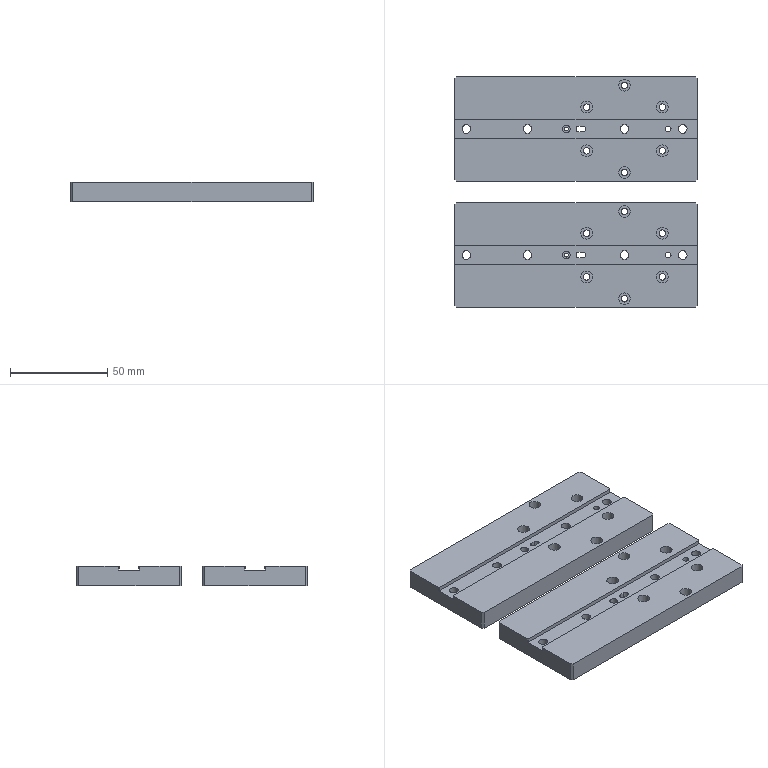Part | 2 solids | 112 faces | box 125 x 119 x 10 mm | volume 124719 mm3 | plane 62 | cylinder 50 | commonest cylinder face diameters 3.4 x12 6 x12 4.5 x8 8 x8 3 x6 2 x2